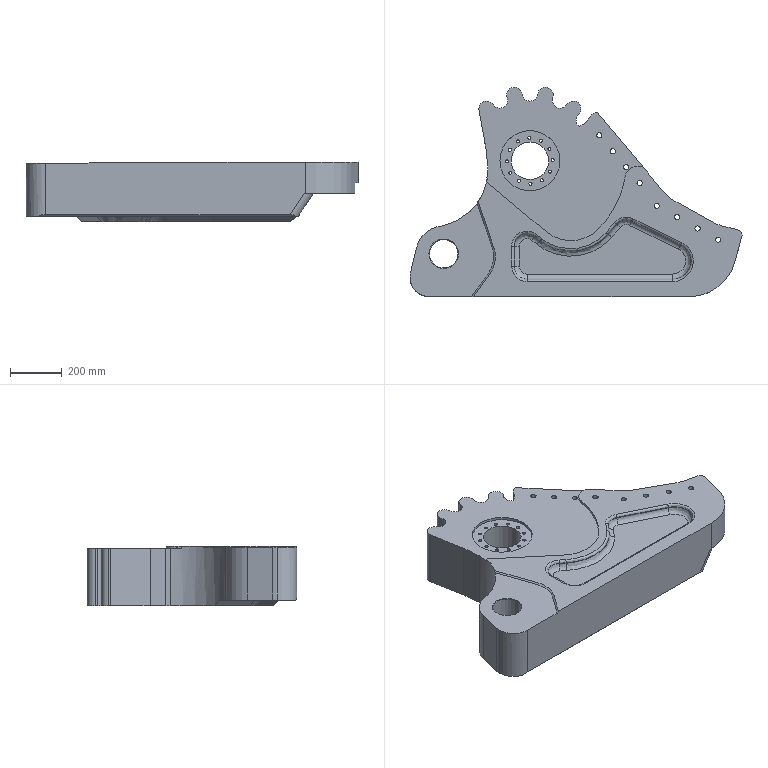Part | SolidWorks | features ICE 6, MoveFace 5, BaseBody 2, Chamfer 1, HoleWzd 1 | 1 solid | 201 faces | box 1278 x 806.277 x 230 mm | volume 104700770 mm3 | cylinder 117 | plane 60 | spline 13 | cone 11 | commonest cylinder face diameters 12 x24 20 x22 60 x11 18 x5 40 x5 9 x4